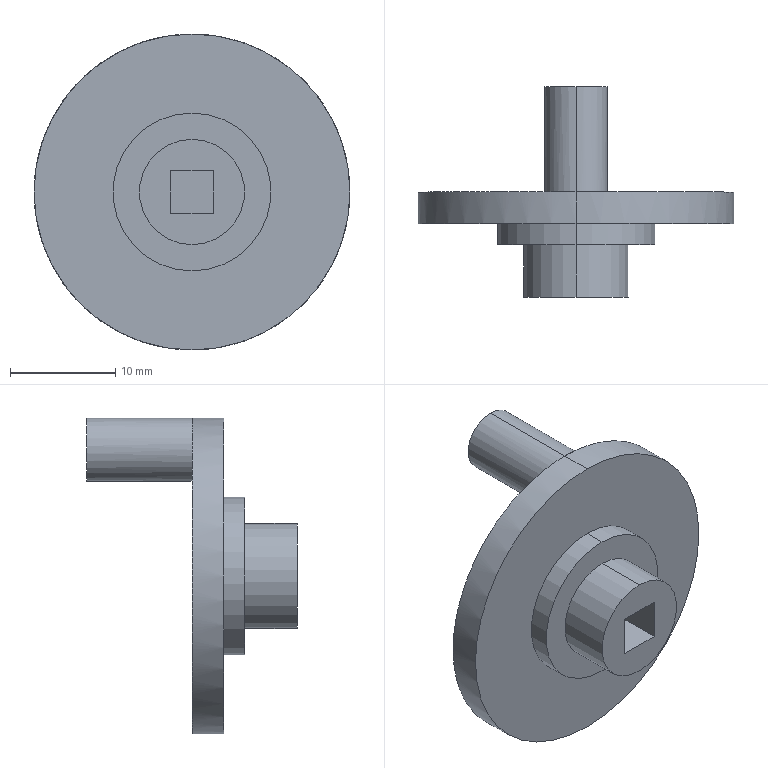Part | SolidWorks | features ICE 4, Extrusion 1 | 1 solid | 18 faces | box 30 x 20 x 30 mm | volume 3069 mm3 | plane 10 | cylinder 8 | commonest cylinder face diameters 6 x2 10 x2 15 x2 30 x2
STEP:
#1=CARTESIAN_POINT('',(0.,-7.,-5.));
#2=VERTEX_POINT('',#1);
#3=CARTESIAN_POINT('',(0.,-7.,5.));
#4=VERTEX_POINT('',#3);
#5=CARTESIAN_POINT('',(0.,-7.,0.));
#6=DIRECTION('',(0.,-1.,0.));
#7=DIRECTION('',(0.,0.,-1.));
#8=AXIS2_PLACEMENT_3D('',#5,#6,#7);
#9=CIRCLE('',#8,5.);
#10=EDGE_CURVE('',#2,#4,#9,.T.);
#11=ORIENTED_EDGE('',*,*,#10,.F.);
#12=CARTESIAN_POINT('',(0.,-2.,-5.));
#13=VERTEX_POINT('',#12);
#14=CARTESIAN_POINT('',(0.,-2.,-5.));
#15=DIRECTION('',(0.,1.,0.));
#16=VECTOR('',#15,1000.);
#17=LINE('',#14,#16);
#18=EDGE_CURVE('',#2,#13,#17,.T.);
#19=ORIENTED_EDGE('',*,*,#18,.T.);
#20=CARTESIAN_POINT('',(0.,-2.,5.));
#21=VERTEX_POINT('',#20);
#22=CARTESIAN_POINT('',(0.,-2.,0.));
#23=DIRECTION('',(0.,-1.,0.));
#24=DIRECTION('',(0.,0.,-1.));
#25=AXIS2_PLACEMENT_3D('',#22,#23,#24);
#26=CIRCLE('',#25,5.);
#27=EDGE_CURVE('',#13,#21,#26,.T.);
#28=ORIENTED_EDGE('',*,*,#27,.T.);
#29=CARTESIAN_POINT('',(0.,-2.,5.));
#30=DIRECTION('',(0.,1.,0.));
#31=VECTOR('',#30,1000.);
#32=LINE('',#29,#31);
#33=EDGE_CURVE('',#4,#21,#32,.T.);
#34=ORIENTED_EDGE('',*,*,#33,.F.);
#35=EDGE_LOOP('',(#11,#19,#28,#34));
#36=FACE_OUTER_BOUND('',#35,.T.);
#37=CARTESIAN_POINT('',(0.,-2.,0.));
#38=DIRECTION('',(0.,1.,0.));
#39=DIRECTION('',(0.,0.,1.));
#40=AXIS2_PLACEMENT_3D('',#37,#38,#39);
#41=CYLINDRICAL_SURFACE('',#40,5.);
#42=ADVANCED_FACE('',(#36),#41,.T.);
#43=CARTESIAN_POINT('',(0.,-2.,-7.5));
#44=VERTEX_POINT('',#43);
#45=CARTESIAN_POINT('',(0.,-2.,7.5));
#46=VERTEX_POINT('',#45);
#47=CARTESIAN_POINT('',(0.,-2.,0.));
#48=DIRECTION('',(0.,-1.,0.));
#49=DIRECTION('',(0.,0.,-1.));
#50=AXIS2_PLACEMENT_3D('',#47,#48,#49);
#51=CIRCLE('',#50,7.5);
#52=EDGE_CURVE('',#44,#46,#51,.T.);
#53=ORIENTED_EDGE('',*,*,#52,.F.);
#54=CARTESIAN_POINT('',(0.,0.,-7.5));
#55=VERTEX_POINT('',#54);
#56=CARTESIAN_POINT('',(0.,-2.,-7.5));
#57=DIRECTION('',(0.,1.,0.));
#58=VECTOR('',#57,1000.);
#59=LINE('',#56,#58);
#60=EDGE_CURVE('',#44,#55,#59,.T.);
#61=ORIENTED_EDGE('',*,*,#60,.T.);
#62=CARTESIAN_POINT('',(0.,0.,7.5));
#63=VERTEX_POINT('',#62);
#64=CARTESIAN_POINT('',(0.,0.,0.));
#65=DIRECTION('',(0.,-1.,0.));
#66=DIRECTION('',(0.,0.,1.));
#67=AXIS2_PLACEMENT_3D('',#64,#65,#66);
#68=CIRCLE('',#67,7.5);
#69=EDGE_CURVE('',#55,#63,#68,.T.);
#70=ORIENTED_EDGE('',*,*,#69,.T.);
#71=CARTESIAN_POINT('',(0.,-2.,7.5));
#72=DIRECTION('',(0.,1.,0.));
#73=VECTOR('',#72,1000.);
#74=LINE('',#71,#73);
#75=EDGE_CURVE('',#46,#63,#74,.T.);
#76=ORIENTED_EDGE('',*,*,#75,.F.);
#77=EDGE_LOOP('',(#53,#61,#70,#76));
#78=FACE_OUTER_BOUND('',#77,.T.);
#79=CARTESIAN_POINT('',(0.,-2.,0.));
#80=DIRECTION('',(0.,1.,0.));
#81=DIRECTION('',(0.,0.,1.));
#82=AXIS2_PLACEMENT_3D('',#79,#80,#81);
#83=CYLINDRICAL_SURFACE('',#82,7.5);
#84=ADVANCED_FACE('',(#78),#83,.T.);
#85=CARTESIAN_POINT('',(0.,13.,15.));
#86=VERTEX_POINT('',#85);
#87=CARTESIAN_POINT('',(0.,13.,9.));
#88=VERTEX_POINT('',#87);
#89=CARTESIAN_POINT('',(0.,13.,12.));
#90=DIRECTION('',(0.,1.,0.));
#91=DIRECTION('',(0.,0.,1.));
#92=AXIS2_PLACEMENT_3D('',#89,#90,#91);
#93=CIRCLE('',#92,3.);
#94=EDGE_CURVE('',#86,#88,#93,.T.);
#95=ORIENTED_EDGE('',*,*,#94,.F.);
#96=CARTESIAN_POINT('',(0.,3.,15.));
#97=VERTEX_POINT('',#96);
#98=CARTESIAN_POINT('',(0.,13.,15.));
#99=DIRECTION('',(0.,-1.,0.));
#100=VECTOR('',#99,1000.);
#101=LINE('',#98,#100);
#102=EDGE_CURVE('',#86,#97,#101,.T.);
#103=ORIENTED_EDGE('',*,*,#102,.T.);
#104=CARTESIAN_POINT('',(0.,3.,9.));
#105=VERTEX_POINT('',#104);
#106=CARTESIAN_POINT('',(0.,3.,12.));
#107=DIRECTION('',(0.,1.,0.));
#108=DIRECTION('',(0.,0.,1.));
#109=AXIS2_PLACEMENT_3D('',#106,#107,#108);
#110=CIRCLE('',#109,3.);
#111=EDGE_CURVE('',#97,#105,#110,.T.);
#112=ORIENTED_EDGE('',*,*,#111,.T.);
#113=CARTESIAN_POINT('',(0.,13.,9.));
#114=DIRECTION('',(0.,-1.,0.));
#115=VECTOR('',#114,1000.);
#116=LINE('',#113,#115);
#117=EDGE_CURVE('',#88,#105,#116,.T.);
#118=ORIENTED_EDGE('',*,*,#117,.F.);
#119=EDGE_LOOP('',(#95,#103,#112,#118));
#120=FACE_OUTER_BOUND('',#119,.T.);
#121=CARTESIAN_POINT('',(0.,13.,12.));
#122=DIRECTION('',(0.,-1.,0.));
#123=DIRECTION('',(0.,0.,-1.));
#124=AXIS2_PLACEMENT_3D('',#121,#122,#123);
#125=CYLINDRICAL_SURFACE('',#124,3.);
#126=ADVANCED_FACE('',(#120),#125,.T.);
#127=CARTESIAN_POINT('',(0.,3.,-15.));
#128=VERTEX_POINT('',#127);
#129=CARTESIAN_POINT('',(0.,3.,0.));
#130=DIRECTION('',(0.,1.,0.));
#131=DIRECTION('',(0.,0.,1.));
#132=AXIS2_PLACEMENT_3D('',#129,#130,#131);
#133=CIRCLE('',#132,15.);
#134=EDGE_CURVE('',#97,#128,#133,.T.);
#135=ORIENTED_EDGE('',*,*,#134,.F.);
#136=CARTESIAN_POINT('',(0.,0.,15.));
#137=VERTEX_POINT('',#136);
#138=CARTESIAN_POINT('',(0.,3.,15.));
#139=DIRECTION('',(0.,-1.,0.));
#140=VECTOR('',#139,1000.);
#141=LINE('',#138,#140);
#142=EDGE_CURVE('',#97,#137,#141,.T.);
#143=ORIENTED_EDGE('',*,*,#142,.T.);
#144=CARTESIAN_POINT('',(0.,0.,-15.));
#145=VERTEX_POINT('',#144);
#146=CARTESIAN_POINT('',(0.,0.,0.));
#147=DIRECTION('',(0.,1.,0.));
#148=DIRECTION('',(0.,0.,1.));
#149=AXIS2_PLACEMENT_3D('',#146,#147,#148);
#150=CIRCLE('',#149,15.);
#151=EDGE_CURVE('',#137,#145,#150,.T.);
#152=ORIENTED_EDGE('',*,*,#151,.T.);
#153=CARTESIAN_POINT('',(0.,3.,-15.));
#154=DIRECTION('',(0.,-1.,0.));
#155=VECTOR('',#154,1000.);
#156=LINE('',#153,#155);
#157=EDGE_CURVE('',#128,#145,#156,.T.);
#158=ORIENTED_EDGE('',*,*,#157,.F.);
#159=EDGE_LOOP('',(#135,#143,#152,#158));
#160=FACE_OUTER_BOUND('',#159,.T.);
#161=CARTESIAN_POINT('',(0.,3.,0.));
#162=DIRECTION('',(0.,-1.,0.));
#163=DIRECTION('',(0.,0.,-1.));
#164=AXIS2_PLACEMENT_3D('',#161,#162,#163);
#165=CYLINDRICAL_SURFACE('',#164,15.);
#166=ADVANCED_FACE('',(#160),#165,.T.);
#167=ORIENTED_EDGE('',*,*,#142,.F.);
#168=CARTESIAN_POINT('',(0.,3.,0.));
#169=DIRECTION('',(0.,1.,0.));
#170=DIRECTION('',(0.,0.,1.));
#171=AXIS2_PLACEMENT_3D('',#168,#169,#170);
#172=CIRCLE('',#171,15.);
#173=EDGE_CURVE('',#128,#97,#172,.T.);
#174=ORIENTED_EDGE('',*,*,#173,.F.);
#175=ORIENTED_EDGE('',*,*,#157,.T.);
#176=CARTESIAN_POINT('',(0.,0.,0.));
#177=DIRECTION('',(0.,1.,0.));
#178=DIRECTION('',(0.,0.,1.));
#179=AXIS2_PLACEMENT_3D('',#176,#177,#178);
#180=CIRCLE('',#179,15.);
#181=EDGE_CURVE('',#145,#137,#180,.T.);
#182=ORIENTED_EDGE('',*,*,#181,.T.);
#183=EDGE_LOOP('',(#167,#174,#175,#182));
#184=FACE_OUTER_BOUND('',#183,.T.);
#185=CARTESIAN_POINT('',(0.,3.,0.));
#186=DIRECTION('',(0.,-1.,0.));
#187=DIRECTION('',(0.,0.,-1.));
#188=AXIS2_PLACEMENT_3D('',#185,#186,#187);
#189=CYLINDRICAL_SURFACE('',#188,15.);
#190=ADVANCED_FACE('',(#184),#189,.T.);
#191=ORIENTED_EDGE('',*,*,#134,.T.);
#192=ORIENTED_EDGE('',*,*,#173,.T.);
#193=CARTESIAN_POINT('',(0.,3.,12.));
#194=DIRECTION('',(0.,1.,0.));
#195=DIRECTION('',(0.,0.,1.));
#196=AXIS2_PLACEMENT_3D('',#193,#194,#195);
#197=CIRCLE('',#196,3.);
#198=EDGE_CURVE('',#105,#97,#197,.T.);
#199=ORIENTED_EDGE('',*,*,#198,.F.);
#200=ORIENTED_EDGE('',*,*,#111,.F.);
#201=EDGE_LOOP('',(#191,#192,#199,#200));
#202=FACE_OUTER_BOUND('',#201,.T.);
#203=CARTESIAN_POINT('',(0.,3.,0.));
#204=DIRECTION('',(0.,1.,0.));
#205=DIRECTION('',(0.,0.,1.));
#206=AXIS2_PLACEMENT_3D('',#203,#204,#205);
#207=PLANE('',#206);
#208=ADVANCED_FACE('',(#202),#207,.T.);
#209=CARTESIAN_POINT('',(0.,0.,0.));
#210=DIRECTION('',(0.,-1.,0.));
#211=DIRECTION('',(0.,0.,1.));
#212=AXIS2_PLACEMENT_3D('',#209,#210,#211);
#213=CIRCLE('',#212,7.5);
#214=EDGE_CURVE('',#63,#55,#213,.T.);
#215=ORIENTED_EDGE('',*,*,#214,.F.);
#216=ORIENTED_EDGE('',*,*,#69,.F.);
#217=EDGE_LOOP('',(#215,#216));
#218=FACE_BOUND('',#217,.T.);
#219=ORIENTED_EDGE('',*,*,#181,.F.);
#220=ORIENTED_EDGE('',*,*,#151,.F.);
#221=EDGE_LOOP('',(#219,#220));
#222=FACE_OUTER_BOUND('',#221,.T.);
#223=CARTESIAN_POINT('',(0.,0.,0.));
#224=DIRECTION('',(0.,1.,0.));
#225=DIRECTION('',(0.,0.,1.));
#226=AXIS2_PLACEMENT_3D('',#223,#224,#225);
#227=PLANE('',#226);
#228=ADVANCED_FACE('',(#218,#222),#227,.F.);
#229=ORIENTED_EDGE('',*,*,#102,.F.);
#230=CARTESIAN_POINT('',(0.,13.,12.));
#231=DIRECTION('',(0.,1.,0.));
#232=DIRECTION('',(0.,0.,1.));
#233=AXIS2_PLACEMENT_3D('',#230,#231,#232);
#234=CIRCLE('',#233,3.);
#235=EDGE_CURVE('',#88,#86,#234,.T.);
#236=ORIENTED_EDGE('',*,*,#235,.F.);
#237=ORIENTED_EDGE('',*,*,#117,.T.);
#238=ORIENTED_EDGE('',*,*,#198,.T.);
#239=EDGE_LOOP('',(#229,#236,#237,#238));
#240=FACE_OUTER_BOUND('',#239,.T.);
#241=CARTESIAN_POINT('',(0.,13.,12.));
#242=DIRECTION('',(0.,-1.,0.));
#243=DIRECTION('',(0.,0.,-1.));
#244=AXIS2_PLACEMENT_3D('',#241,#242,#243);
#245=CYLINDRICAL_SURFACE('',#244,3.);
#246=ADVANCED_FACE('',(#240),#245,.T.);
#247=ORIENTED_EDGE('',*,*,#235,.T.);
#248=ORIENTED_EDGE('',*,*,#94,.T.);
#249=EDGE_LOOP('',(#247,#248));
#250=FACE_OUTER_BOUND('',#249,.T.);
#251=CARTESIAN_POINT('',(0.,13.,12.));
#252=DIRECTION('',(0.,1.,0.));
#253=DIRECTION('',(0.,0.,1.));
#254=AXIS2_PLACEMENT_3D('',#251,#252,#253);
#255=PLANE('',#254);
#256=ADVANCED_FACE('',(#250),#255,.T.);
#257=ORIENTED_EDGE('',*,*,#60,.F.);
#258=CARTESIAN_POINT('',(0.,-2.,0.));
#259=DIRECTION('',(0.,-1.,0.));
#260=DIRECTION('',(0.,0.,-1.));
#261=AXIS2_PLACEMENT_3D('',#258,#259,#260);
#262=CIRCLE('',#261,7.5);
#263=EDGE_CURVE('',#46,#44,#262,.T.);
#264=ORIENTED_EDGE('',*,*,#263,.F.);
#265=ORIENTED_EDGE('',*,*,#75,.T.);
#266=ORIENTED_EDGE('',*,*,#214,.T.);
#267=EDGE_LOOP('',(#257,#264,#265,#266));
#268=FACE_OUTER_BOUND('',#267,.T.);
#269=CARTESIAN_POINT('',(0.,-2.,0.));
#270=DIRECTION('',(0.,1.,0.));
#271=DIRECTION('',(0.,0.,1.));
#272=AXIS2_PLACEMENT_3D('',#269,#270,#271);
#273=CYLINDRICAL_SURFACE('',#272,7.5);
#274=ADVANCED_FACE('',(#268),#273,.T.);
#275=CARTESIAN_POINT('',(0.,-2.,0.));
#276=DIRECTION('',(0.,-1.,0.));
#277=DIRECTION('',(0.,0.,-1.));
#278=AXIS2_PLACEMENT_3D('',#275,#276,#277);
#279=CIRCLE('',#278,5.);
#280=EDGE_CURVE('',#21,#13,#279,.T.);
#281=ORIENTED_EDGE('',*,*,#280,.F.);
#282=ORIENTED_EDGE('',*,*,#27,.F.);
#283=EDGE_LOOP('',(#281,#282));
#284=FACE_BOUND('',#283,.T.);
#285=ORIENTED_EDGE('',*,*,#263,.T.);
#286=ORIENTED_EDGE('',*,*,#52,.T.);
#287=EDGE_LOOP('',(#285,#286));
#288=FACE_OUTER_BOUND('',#287,.T.);
#289=CARTESIAN_POINT('',(0.,-2.,0.));
#290=DIRECTION('',(0.,-1.,0.));
#291=DIRECTION('',(0.,0.,-1.));
#292=AXIS2_PLACEMENT_3D('',#289,#290,#291);
#293=PLANE('',#292);
#294=ADVANCED_FACE('',(#284,#288),#293,.T.);
#295=CARTESIAN_POINT('',(2.,-2.,-2.));
#296=VERTEX_POINT('',#295);
#297=CARTESIAN_POINT('',(2.,-2.,2.));
#298=VERTEX_POINT('',#297);
#299=CARTESIAN_POINT('',(2.,-2.,-2.));
#300=DIRECTION('',(0.,0.,1.));
#301=VECTOR('',#300,1000.);
#302=LINE('',#299,#301);
#303=EDGE_CURVE('',#296,#298,#302,.T.);
#304=ORIENTED_EDGE('',*,*,#303,.T.);
#305=CARTESIAN_POINT('',(-2.,-2.,2.));
#306=VERTEX_POINT('',#305);
#307=CARTESIAN_POINT('',(-2.,-2.,2.));
#308=DIRECTION('',(-1.,0.,0.));
#309=VECTOR('',#308,1000.);
#310=LINE('',#307,#309);
#311=EDGE_CURVE('',#298,#306,#310,.T.);
#312=ORIENTED_EDGE('',*,*,#311,.T.);
#313=CARTESIAN_POINT('',(-2.,-2.,-2.));
#314=VERTEX_POINT('',#313);
#315=CARTESIAN_POINT('',(-2.,-2.,-2.));
#316=DIRECTION('',(0.,0.,-1.));
#317=VECTOR('',#316,1000.);
#318=LINE('',#315,#317);
#319=EDGE_CURVE('',#306,#314,#318,.T.);
#320=ORIENTED_EDGE('',*,*,#319,.T.);
#321=CARTESIAN_POINT('',(-2.,-2.,-2.));
#322=DIRECTION('',(1.,0.,0.));
#323=VECTOR('',#322,1000.);
#324=LINE('',#321,#323);
#325=EDGE_CURVE('',#314,#296,#324,.T.);
#326=ORIENTED_EDGE('',*,*,#325,.T.);
#327=EDGE_LOOP('',(#304,#312,#320,#326));
#328=FACE_OUTER_BOUND('',#327,.T.);
#329=CARTESIAN_POINT('',(0.,-2.,0.));
#330=DIRECTION('',(0.,-1.,0.));
#331=DIRECTION('',(0.,0.,-1.));
#332=AXIS2_PLACEMENT_3D('',#329,#330,#331);
#333=PLANE('',#332);
#334=ADVANCED_FACE('',(#328),#333,.T.);
#335=ORIENTED_EDGE('',*,*,#319,.F.);
#336=CARTESIAN_POINT('',(-2.,-7.,2.));
#337=VERTEX_POINT('',#336);
#338=CARTESIAN_POINT('',(-2.,-7.,2.));
#339=DIRECTION('',(0.,1.,0.));
#340=VECTOR('',#339,1000.);
#341=LINE('',#338,#340);
#342=EDGE_CURVE('',#337,#306,#341,.T.);
#343=ORIENTED_EDGE('',*,*,#342,.F.);
#344=CARTESIAN_POINT('',(-2.,-7.,-2.));
#345=VERTEX_POINT('',#344);
#346=CARTESIAN_POINT('',(-2.,-7.,-2.));
#347=DIRECTION('',(0.,0.,-1.));
#348=VECTOR('',#347,1000.);
#349=LINE('',#346,#348);
#350=EDGE_CURVE('',#337,#345,#349,.T.);
#351=ORIENTED_EDGE('',*,*,#350,.T.);
#352=CARTESIAN_POINT('',(-2.,-7.,-2.));
#353=DIRECTION('',(0.,1.,0.));
#354=VECTOR('',#353,1000.);
#355=LINE('',#352,#354);
#356=EDGE_CURVE('',#345,#314,#355,.T.);
#357=ORIENTED_EDGE('',*,*,#356,.T.);
#358=EDGE_LOOP('',(#335,#343,#351,#357));
#359=FACE_OUTER_BOUND('',#358,.T.);
#360=CARTESIAN_POINT('',(-2.,-7.,-2.));
#361=DIRECTION('',(1.,0.,0.));
#362=DIRECTION('',(0.,0.,-1.));
#363=AXIS2_PLACEMENT_3D('',#360,#361,#362);
#364=PLANE('',#363);
#365=ADVANCED_FACE('',(#359),#364,.T.);
#366=ORIENTED_EDGE('',*,*,#325,.F.);
#367=ORIENTED_EDGE('',*,*,#356,.F.);
#368=CARTESIAN_POINT('',(2.,-7.,-2.));
#369=VERTEX_POINT('',#368);
#370=CARTESIAN_POINT('',(-2.,-7.,-2.));
#371=DIRECTION('',(1.,0.,0.));
#372=VECTOR('',#371,1000.);
#373=LINE('',#370,#372);
#374=EDGE_CURVE('',#345,#369,#373,.T.);
#375=ORIENTED_EDGE('',*,*,#374,.T.);
#376=CARTESIAN_POINT('',(2.,-7.,-2.));
#377=DIRECTION('',(0.,1.,0.));
#378=VECTOR('',#377,1000.);
#379=LINE('',#376,#378);
#380=EDGE_CURVE('',#369,#296,#379,.T.);
#381=ORIENTED_EDGE('',*,*,#380,.T.);
#382=EDGE_LOOP('',(#366,#367,#375,#381));
#383=FACE_OUTER_BOUND('',#382,.T.);
#384=CARTESIAN_POINT('',(-2.,-7.,-2.));
#385=DIRECTION('',(0.,0.,1.));
#386=DIRECTION('',(1.,0.,0.));
#387=AXIS2_PLACEMENT_3D('',#384,#385,#386);
#388=PLANE('',#387);
#389=ADVANCED_FACE('',(#383),#388,.T.);
#390=ORIENTED_EDGE('',*,*,#303,.F.);
#391=ORIENTED_EDGE('',*,*,#380,.F.);
#392=CARTESIAN_POINT('',(2.,-7.,2.));
#393=VERTEX_POINT('',#392);
#394=CARTESIAN_POINT('',(2.,-7.,-2.));
#395=DIRECTION('',(0.,0.,1.));
#396=VECTOR('',#395,1000.);
#397=LINE('',#394,#396);
#398=EDGE_CURVE('',#369,#393,#397,.T.);
#399=ORIENTED_EDGE('',*,*,#398,.T.);
#400=CARTESIAN_POINT('',(2.,-7.,2.));
#401=DIRECTION('',(0.,1.,0.));
#402=VECTOR('',#401,1000.);
#403=LINE('',#400,#402);
#404=EDGE_CURVE('',#393,#298,#403,.T.);
#405=ORIENTED_EDGE('',*,*,#404,.T.);
#406=EDGE_LOOP('',(#390,#391,#399,#405));
#407=FACE_OUTER_BOUND('',#406,.T.);
#408=CARTESIAN_POINT('',(2.,-7.,-2.));
#409=DIRECTION('',(-1.,0.,0.));
#410=DIRECTION('',(0.,0.,1.));
#411=AXIS2_PLACEMENT_3D('',#408,#409,#410);
#412=PLANE('',#411);
#413=ADVANCED_FACE('',(#407),#412,.T.);
#414=ORIENTED_EDGE('',*,*,#311,.F.);
#415=ORIENTED_EDGE('',*,*,#404,.F.);
#416=CARTESIAN_POINT('',(-2.,-7.,2.));
#417=DIRECTION('',(-1.,0.,0.));
#418=VECTOR('',#417,1000.);
#419=LINE('',#416,#418);
#420=EDGE_CURVE('',#393,#337,#419,.T.);
#421=ORIENTED_EDGE('',*,*,#420,.T.);
#422=ORIENTED_EDGE('',*,*,#342,.T.);
#423=EDGE_LOOP('',(#414,#415,#421,#422));
#424=FACE_OUTER_BOUND('',#423,.T.);
#425=CARTESIAN_POINT('',(-2.,-7.,2.));
#426=DIRECTION('',(0.,0.,-1.));
#427=DIRECTION('',(-1.,0.,0.));
#428=AXIS2_PLACEMENT_3D('',#425,#426,#427);
#429=PLANE('',#428);
#430=ADVANCED_FACE('',(#424),#429,.T.);
#431=CARTESIAN_POINT('',(0.,-7.,0.));
#432=DIRECTION('',(0.,-1.,0.));
#433=DIRECTION('',(0.,0.,-1.));
#434=AXIS2_PLACEMENT_3D('',#431,#432,#433);
#435=CIRCLE('',#434,5.);
#436=EDGE_CURVE('',#4,#2,#435,.T.);
#437=ORIENTED_EDGE('',*,*,#436,.T.);
#438=ORIENTED_EDGE('',*,*,#10,.T.);
#439=EDGE_LOOP('',(#437,#438));
#440=FACE_OUTER_BOUND('',#439,.T.);
#441=ORIENTED_EDGE('',*,*,#420,.F.);
#442=ORIENTED_EDGE('',*,*,#398,.F.);
#443=ORIENTED_EDGE('',*,*,#374,.F.);
#444=ORIENTED_EDGE('',*,*,#350,.F.);
#445=EDGE_LOOP('',(#441,#442,#443,#444));
#446=FACE_BOUND('',#445,.T.);
#447=CARTESIAN_POINT('',(0.,-7.,0.));
#448=DIRECTION('',(0.,-1.,0.));
#449=DIRECTION('',(0.,0.,-1.));
#450=AXIS2_PLACEMENT_3D('',#447,#448,#449);
#451=PLANE('',#450);
#452=ADVANCED_FACE('',(#440,#446),#451,.T.);
#453=ORIENTED_EDGE('',*,*,#18,.F.);
#454=ORIENTED_EDGE('',*,*,#436,.F.);
#455=ORIENTED_EDGE('',*,*,#33,.T.);
#456=ORIENTED_EDGE('',*,*,#280,.T.);
#457=EDGE_LOOP('',(#453,#454,#455,#456));
#458=FACE_OUTER_BOUND('',#457,.T.);
#459=CARTESIAN_POINT('',(0.,-2.,0.));
#460=DIRECTION('',(0.,1.,0.));
#461=DIRECTION('',(0.,0.,1.));
#462=AXIS2_PLACEMENT_3D('',#459,#460,#461);
#463=CYLINDRICAL_SURFACE('',#462,5.);
#464=ADVANCED_FACE('',(#458),#463,.T.);
#465=CLOSED_SHELL('',(#42,#84,#126,#166,#190,#208,#228,#246,#256,#274,#294,#334,#365,#389,#413,#430,#452,#464));
#466=MANIFOLD_SOLID_BREP('',#465);
#467=CARTESIAN_POINT('',(0.,0.,0.));
#468=DIRECTION('',(0.,0.,1.));
#469=DIRECTION('',(1.,0.,0.));
#470=AXIS2_PLACEMENT_3D('',#467,#468,#469);
#471=(LENGTH_UNIT()NAMED_UNIT(*)SI_UNIT(.MILLI.,.METRE.));
#472=UNCERTAINTY_MEASURE_WITH_UNIT(LENGTH_MEASURE(0.00001),#471,'','');
#473=(NAMED_UNIT(*)PLANE_ANGLE_UNIT()SI_UNIT($,.RADIAN.));
#474=(NAMED_UNIT(*)SI_UNIT($,.STERADIAN.)SOLID_ANGLE_UNIT());
#475=(GEOMETRIC_REPRESENTATION_CONTEXT(3)GLOBAL_UNCERTAINTY_ASSIGNED_CONTEXT((#472))GLOBAL_UNIT_ASSIGNED_CONTEXT((#471,#473,#474))REPRESENTATION_CONTEXT('',''));
#476=ADVANCED_BREP_SHAPE_REPRESENTATION('',(#466,#470),#475);